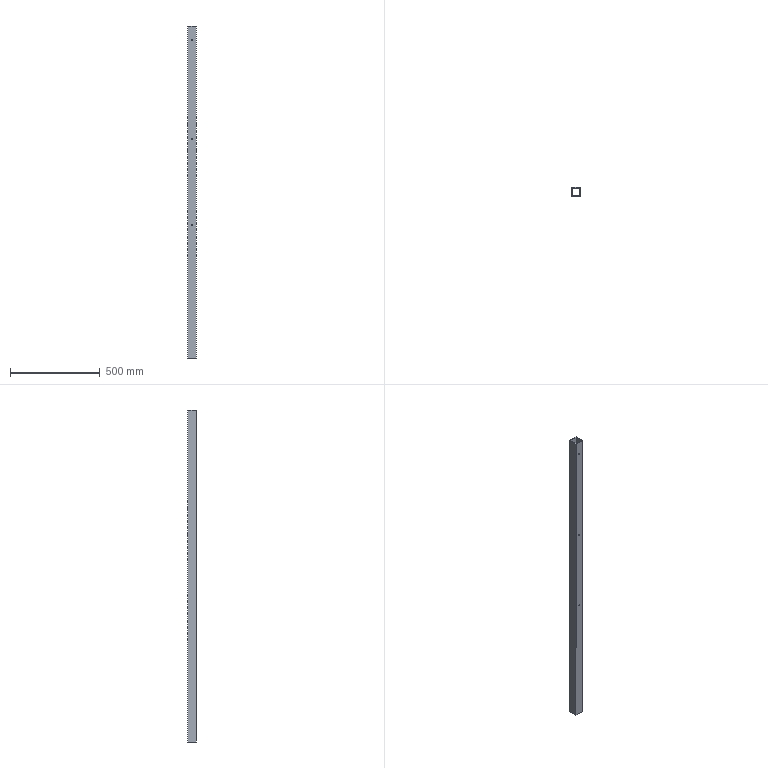Part | NX | features solid 2 | 1 solid | 16 faces | box 50 x 50 x 1848 mm | volume 1662776 mm3 | plane 10 | cylinder 6 | commonest cylinder face diameters 6 x6
STEP:
#1=CARTESIAN_POINT('',(-355.,5.,132.));
#2=VERTEX_POINT('',#1);
#3=CARTESIAN_POINT('',(-355.,0.,132.));
#4=VERTEX_POINT('',#3);
#5=CARTESIAN_POINT('',(-355.,1811.381,132.));
#6=DIRECTION('',(0.,-1.,0.));
#7=VECTOR('',#6,1000.);
#8=LINE('',#5,#7);
#9=EDGE_CURVE('',#2,#4,#8,.T.);
#10=ORIENTED_EDGE('',*,*,#9,.F.);
#11=CARTESIAN_POINT('',(-355.,5.,138.));
#12=VERTEX_POINT('',#11);
#13=CARTESIAN_POINT('',(-355.,5.,135.));
#14=DIRECTION('',(0.,1.,0.));
#15=DIRECTION('',(0.,0.,-1.));
#16=AXIS2_PLACEMENT_3D('',#13,#14,#15);
#17=CIRCLE('',#16,3.);
#18=EDGE_CURVE('',#2,#12,#17,.T.);
#19=ORIENTED_EDGE('',*,*,#18,.T.);
#20=CARTESIAN_POINT('',(-355.,0.,138.));
#21=VERTEX_POINT('',#20);
#22=CARTESIAN_POINT('',(-355.,1811.381,138.));
#23=DIRECTION('',(0.,-1.,0.));
#24=VECTOR('',#23,1000.);
#25=LINE('',#22,#24);
#26=EDGE_CURVE('',#21,#12,#25,.F.);
#27=ORIENTED_EDGE('',*,*,#26,.F.);
#28=CARTESIAN_POINT('',(-355.,0.,135.));
#29=DIRECTION('',(0.,-1.,0.));
#30=DIRECTION('',(0.,0.,1.));
#31=AXIS2_PLACEMENT_3D('',#28,#29,#30);
#32=CIRCLE('',#31,3.);
#33=EDGE_CURVE('',#21,#4,#32,.T.);
#34=ORIENTED_EDGE('',*,*,#33,.T.);
#35=EDGE_LOOP('',(#10,#19,#27,#34));
#36=FACE_BOUND('',#35,.T.);
#37=CARTESIAN_POINT('',(-355.,1811.381,135.));
#38=DIRECTION('',(0.,-1.,0.));
#39=DIRECTION('',(0.,0.,1.));
#40=AXIS2_PLACEMENT_3D('',#37,#38,#39);
#41=CYLINDRICAL_SURFACE('',#40,3.);
#42=ADVANCED_FACE('',(#36),#41,.F.);
#43=CARTESIAN_POINT('',(-355.,5.,612.));
#44=VERTEX_POINT('',#43);
#45=CARTESIAN_POINT('',(-355.,0.,612.));
#46=VERTEX_POINT('',#45);
#47=CARTESIAN_POINT('',(-355.,1811.381,612.));
#48=DIRECTION('',(0.,-1.,0.));
#49=VECTOR('',#48,1000.);
#50=LINE('',#47,#49);
#51=EDGE_CURVE('',#44,#46,#50,.T.);
#52=ORIENTED_EDGE('',*,*,#51,.F.);
#53=CARTESIAN_POINT('',(-355.,5.,618.));
#54=VERTEX_POINT('',#53);
#55=CARTESIAN_POINT('',(-355.,5.,615.));
#56=DIRECTION('',(0.,1.,0.));
#57=DIRECTION('',(0.,0.,-1.));
#58=AXIS2_PLACEMENT_3D('',#55,#56,#57);
#59=CIRCLE('',#58,3.);
#60=EDGE_CURVE('',#44,#54,#59,.T.);
#61=ORIENTED_EDGE('',*,*,#60,.T.);
#62=CARTESIAN_POINT('',(-355.,0.,618.));
#63=VERTEX_POINT('',#62);
#64=CARTESIAN_POINT('',(-355.,1811.381,618.));
#65=DIRECTION('',(0.,-1.,0.));
#66=VECTOR('',#65,1000.);
#67=LINE('',#64,#66);
#68=EDGE_CURVE('',#63,#54,#67,.F.);
#69=ORIENTED_EDGE('',*,*,#68,.F.);
#70=CARTESIAN_POINT('',(-355.,0.,615.));
#71=DIRECTION('',(0.,-1.,0.));
#72=DIRECTION('',(0.,0.,1.));
#73=AXIS2_PLACEMENT_3D('',#70,#71,#72);
#74=CIRCLE('',#73,3.);
#75=EDGE_CURVE('',#63,#46,#74,.T.);
#76=ORIENTED_EDGE('',*,*,#75,.T.);
#77=EDGE_LOOP('',(#52,#61,#69,#76));
#78=FACE_BOUND('',#77,.T.);
#79=CARTESIAN_POINT('',(-355.,1811.381,615.));
#80=DIRECTION('',(0.,-1.,0.));
#81=DIRECTION('',(0.,0.,1.));
#82=AXIS2_PLACEMENT_3D('',#79,#80,#81);
#83=CYLINDRICAL_SURFACE('',#82,3.);
#84=ADVANCED_FACE('',(#78),#83,.F.);
#85=CARTESIAN_POINT('',(-355.,0.,1162.));
#86=VERTEX_POINT('',#85);
#87=CARTESIAN_POINT('',(-355.,5.,1162.));
#88=VERTEX_POINT('',#87);
#89=CARTESIAN_POINT('',(-355.,1811.381,1162.));
#90=DIRECTION('',(0.,-1.,0.));
#91=VECTOR('',#90,1000.);
#92=LINE('',#89,#91);
#93=EDGE_CURVE('',#86,#88,#92,.F.);
#94=ORIENTED_EDGE('',*,*,#93,.T.);
#95=CARTESIAN_POINT('',(-355.,5.,1168.));
#96=VERTEX_POINT('',#95);
#97=CARTESIAN_POINT('',(-355.,5.,1165.));
#98=DIRECTION('',(0.,1.,0.));
#99=DIRECTION('',(0.,0.,-1.));
#100=AXIS2_PLACEMENT_3D('',#97,#98,#99);
#101=CIRCLE('',#100,3.);
#102=EDGE_CURVE('',#88,#96,#101,.T.);
#103=ORIENTED_EDGE('',*,*,#102,.T.);
#104=CARTESIAN_POINT('',(-355.,0.,1168.));
#105=VERTEX_POINT('',#104);
#106=CARTESIAN_POINT('',(-355.,1811.381,1168.));
#107=DIRECTION('',(0.,-1.,0.));
#108=VECTOR('',#107,1000.);
#109=LINE('',#106,#108);
#110=EDGE_CURVE('',#96,#105,#109,.T.);
#111=ORIENTED_EDGE('',*,*,#110,.T.);
#112=CARTESIAN_POINT('',(-355.,0.,1165.));
#113=DIRECTION('',(0.,-1.,0.));
#114=DIRECTION('',(0.,0.,1.));
#115=AXIS2_PLACEMENT_3D('',#112,#113,#114);
#116=CIRCLE('',#115,3.);
#117=EDGE_CURVE('',#105,#86,#116,.T.);
#118=ORIENTED_EDGE('',*,*,#117,.T.);
#119=EDGE_LOOP('',(#94,#103,#111,#118));
#120=FACE_BOUND('',#119,.T.);
#121=CARTESIAN_POINT('',(-355.,1811.381,1165.));
#122=DIRECTION('',(0.,-1.,0.));
#123=DIRECTION('',(0.,0.,1.));
#124=AXIS2_PLACEMENT_3D('',#121,#122,#123);
#125=CYLINDRICAL_SURFACE('',#124,3.);
#126=ADVANCED_FACE('',(#120),#125,.F.);
#127=CARTESIAN_POINT('',(-380.,50.,-603.));
#128=VERTEX_POINT('',#127);
#129=CARTESIAN_POINT('',(-380.,50.,1245.));
#130=VERTEX_POINT('',#129);
#131=CARTESIAN_POINT('',(-380.,50.,-495.));
#132=DIRECTION('',(0.,0.,1.));
#133=VECTOR('',#132,1000.);
#134=LINE('',#131,#133);
#135=EDGE_CURVE('',#128,#130,#134,.T.);
#136=ORIENTED_EDGE('',*,*,#135,.T.);
#137=CARTESIAN_POINT('',(-330.,50.,1245.));
#138=VERTEX_POINT('',#137);
#139=CARTESIAN_POINT('',(-380.,50.,1245.));
#140=DIRECTION('',(-1.,0.,0.));
#141=VECTOR('',#140,1000.);
#142=LINE('',#139,#141);
#143=EDGE_CURVE('',#138,#130,#142,.T.);
#144=ORIENTED_EDGE('',*,*,#143,.F.);
#145=CARTESIAN_POINT('',(-330.,50.,-603.));
#146=VERTEX_POINT('',#145);
#147=CARTESIAN_POINT('',(-330.,50.,-495.));
#148=DIRECTION('',(0.,0.,-1.));
#149=VECTOR('',#148,1000.);
#150=LINE('',#147,#149);
#151=EDGE_CURVE('',#138,#146,#150,.T.);
#152=ORIENTED_EDGE('',*,*,#151,.T.);
#153=CARTESIAN_POINT('',(-380.,50.,-603.));
#154=DIRECTION('',(-1.,0.,0.));
#155=VECTOR('',#154,1000.);
#156=LINE('',#153,#155);
#157=EDGE_CURVE('',#146,#128,#156,.T.);
#158=ORIENTED_EDGE('',*,*,#157,.T.);
#159=EDGE_LOOP('',(#136,#144,#152,#158));
#160=FACE_BOUND('',#159,.T.);
#161=CARTESIAN_POINT('',(-380.,50.,-495.));
#162=DIRECTION('',(0.,-1.,0.));
#163=DIRECTION('',(-1.,0.,0.));
#164=AXIS2_PLACEMENT_3D('',#161,#162,#163);
#165=PLANE('',#164);
#166=ADVANCED_FACE('',(#160),#165,.F.);
#167=CARTESIAN_POINT('',(-375.,45.,1245.));
#168=VERTEX_POINT('',#167);
#169=CARTESIAN_POINT('',(-335.,45.,1245.));
#170=VERTEX_POINT('',#169);
#171=CARTESIAN_POINT('',(-330.,45.,1245.));
#172=DIRECTION('',(1.,0.,0.));
#173=VECTOR('',#172,1000.);
#174=LINE('',#171,#173);
#175=EDGE_CURVE('',#168,#170,#174,.T.);
#176=ORIENTED_EDGE('',*,*,#175,.F.);
#177=CARTESIAN_POINT('',(-375.,45.,-603.));
#178=VERTEX_POINT('',#177);
#179=CARTESIAN_POINT('',(-375.,45.,-495.));
#180=DIRECTION('',(0.,0.,1.));
#181=VECTOR('',#180,1000.);
#182=LINE('',#179,#181);
#183=EDGE_CURVE('',#178,#168,#182,.T.);
#184=ORIENTED_EDGE('',*,*,#183,.F.);
#185=CARTESIAN_POINT('',(-335.,45.,-603.));
#186=VERTEX_POINT('',#185);
#187=CARTESIAN_POINT('',(-330.,45.,-603.));
#188=DIRECTION('',(1.,0.,0.));
#189=VECTOR('',#188,1000.);
#190=LINE('',#187,#189);
#191=EDGE_CURVE('',#178,#186,#190,.T.);
#192=ORIENTED_EDGE('',*,*,#191,.T.);
#193=CARTESIAN_POINT('',(-335.,45.,-495.));
#194=DIRECTION('',(0.,0.,-1.));
#195=VECTOR('',#194,1000.);
#196=LINE('',#193,#195);
#197=EDGE_CURVE('',#170,#186,#196,.T.);
#198=ORIENTED_EDGE('',*,*,#197,.F.);
#199=EDGE_LOOP('',(#176,#184,#192,#198));
#200=FACE_BOUND('',#199,.T.);
#201=CARTESIAN_POINT('',(-375.,45.,-495.));
#202=DIRECTION('',(0.,-1.,0.));
#203=DIRECTION('',(-1.,0.,0.));
#204=AXIS2_PLACEMENT_3D('',#201,#202,#203);
#205=PLANE('',#204);
#206=ADVANCED_FACE('',(#200),#205,.T.);
#207=CARTESIAN_POINT('',(-380.,0.,-603.));
#208=VERTEX_POINT('',#207);
#209=CARTESIAN_POINT('',(-380.,0.,1245.));
#210=VERTEX_POINT('',#209);
#211=CARTESIAN_POINT('',(-380.,0.,1245.));
#212=DIRECTION('',(0.,0.,1.));
#213=VECTOR('',#212,1000.);
#214=LINE('',#211,#213);
#215=EDGE_CURVE('',#208,#210,#214,.T.);
#216=ORIENTED_EDGE('',*,*,#215,.T.);
#217=CARTESIAN_POINT('',(-380.,0.,1245.));
#218=DIRECTION('',(0.,-1.,0.));
#219=VECTOR('',#218,1000.);
#220=LINE('',#217,#219);
#221=EDGE_CURVE('',#130,#210,#220,.T.);
#222=ORIENTED_EDGE('',*,*,#221,.F.);
#223=ORIENTED_EDGE('',*,*,#135,.F.);
#224=CARTESIAN_POINT('',(-380.,0.,-603.));
#225=DIRECTION('',(0.,-1.,0.));
#226=VECTOR('',#225,1000.);
#227=LINE('',#224,#226);
#228=EDGE_CURVE('',#128,#208,#227,.T.);
#229=ORIENTED_EDGE('',*,*,#228,.T.);
#230=EDGE_LOOP('',(#216,#222,#223,#229));
#231=FACE_BOUND('',#230,.T.);
#232=CARTESIAN_POINT('',(-380.,0.,1245.));
#233=DIRECTION('',(1.,0.,0.));
#234=DIRECTION('',(0.,-1.,0.));
#235=AXIS2_PLACEMENT_3D('',#232,#233,#234);
#236=PLANE('',#235);
#237=ADVANCED_FACE('',(#231),#236,.F.);
#238=ORIENTED_EDGE('',*,*,#151,.F.);
#239=CARTESIAN_POINT('',(-330.,0.,1245.));
#240=VERTEX_POINT('',#239);
#241=CARTESIAN_POINT('',(-330.,0.,1245.));
#242=DIRECTION('',(0.,1.,0.));
#243=VECTOR('',#242,1000.);
#244=LINE('',#241,#243);
#245=EDGE_CURVE('',#240,#138,#244,.T.);
#246=ORIENTED_EDGE('',*,*,#245,.F.);
#247=CARTESIAN_POINT('',(-330.,0.,-603.));
#248=VERTEX_POINT('',#247);
#249=CARTESIAN_POINT('',(-330.,0.,-495.));
#250=DIRECTION('',(0.,0.,-1.));
#251=VECTOR('',#250,1000.);
#252=LINE('',#249,#251);
#253=EDGE_CURVE('',#240,#248,#252,.T.);
#254=ORIENTED_EDGE('',*,*,#253,.T.);
#255=CARTESIAN_POINT('',(-330.,0.,-603.));
#256=DIRECTION('',(0.,1.,0.));
#257=VECTOR('',#256,1000.);
#258=LINE('',#255,#257);
#259=EDGE_CURVE('',#248,#146,#258,.T.);
#260=ORIENTED_EDGE('',*,*,#259,.T.);
#261=EDGE_LOOP('',(#238,#246,#254,#260));
#262=FACE_BOUND('',#261,.T.);
#263=CARTESIAN_POINT('',(-330.,0.,-495.));
#264=DIRECTION('',(-1.,0.,0.));
#265=DIRECTION('',(0.,0.,1.));
#266=AXIS2_PLACEMENT_3D('',#263,#264,#265);
#267=PLANE('',#266);
#268=ADVANCED_FACE('',(#262),#267,.F.);
#269=CARTESIAN_POINT('',(-335.,5.,-603.));
#270=VERTEX_POINT('',#269);
#271=CARTESIAN_POINT('',(-335.,0.,-603.));
#272=DIRECTION('',(0.,-1.,0.));
#273=VECTOR('',#272,1000.);
#274=LINE('',#271,#273);
#275=EDGE_CURVE('',#186,#270,#274,.T.);
#276=ORIENTED_EDGE('',*,*,#275,.F.);
#277=ORIENTED_EDGE('',*,*,#191,.F.);
#278=CARTESIAN_POINT('',(-375.,5.,-603.));
#279=VERTEX_POINT('',#278);
#280=CARTESIAN_POINT('',(-375.,0.,-603.));
#281=DIRECTION('',(0.,1.,0.));
#282=VECTOR('',#281,1000.);
#283=LINE('',#280,#282);
#284=EDGE_CURVE('',#279,#178,#283,.T.);
#285=ORIENTED_EDGE('',*,*,#284,.F.);
#286=CARTESIAN_POINT('',(-330.,5.,-603.));
#287=DIRECTION('',(-1.,0.,0.));
#288=VECTOR('',#287,1000.);
#289=LINE('',#286,#288);
#290=EDGE_CURVE('',#270,#279,#289,.T.);
#291=ORIENTED_EDGE('',*,*,#290,.F.);
#292=EDGE_LOOP('',(#276,#277,#285,#291));
#293=FACE_BOUND('',#292,.T.);
#294=ORIENTED_EDGE('',*,*,#228,.F.);
#295=ORIENTED_EDGE('',*,*,#157,.F.);
#296=ORIENTED_EDGE('',*,*,#259,.F.);
#297=CARTESIAN_POINT('',(-330.,0.,-603.));
#298=DIRECTION('',(-1.,0.,0.));
#299=VECTOR('',#298,1000.);
#300=LINE('',#297,#299);
#301=EDGE_CURVE('',#248,#208,#300,.T.);
#302=ORIENTED_EDGE('',*,*,#301,.T.);
#303=EDGE_LOOP('',(#294,#295,#296,#302));
#304=FACE_BOUND('',#303,.T.);
#305=CARTESIAN_POINT('',(-330.,0.,-603.));
#306=DIRECTION('',(0.,0.,1.));
#307=DIRECTION('',(0.,-1.,0.));
#308=AXIS2_PLACEMENT_3D('',#305,#306,#307);
#309=PLANE('',#308);
#310=ADVANCED_FACE('',(#293,#304),#309,.F.);
#311=CARTESIAN_POINT('',(-375.,5.,1245.));
#312=VERTEX_POINT('',#311);
#313=CARTESIAN_POINT('',(-375.,0.,1245.));
#314=DIRECTION('',(0.,1.,0.));
#315=VECTOR('',#314,1000.);
#316=LINE('',#313,#315);
#317=EDGE_CURVE('',#312,#168,#316,.T.);
#318=ORIENTED_EDGE('',*,*,#317,.F.);
#319=CARTESIAN_POINT('',(-375.,5.,1245.));
#320=DIRECTION('',(0.,0.,1.));
#321=VECTOR('',#320,1000.);
#322=LINE('',#319,#321);
#323=EDGE_CURVE('',#279,#312,#322,.T.);
#324=ORIENTED_EDGE('',*,*,#323,.F.);
#325=ORIENTED_EDGE('',*,*,#284,.T.);
#326=ORIENTED_EDGE('',*,*,#183,.T.);
#327=EDGE_LOOP('',(#318,#324,#325,#326));
#328=FACE_BOUND('',#327,.T.);
#329=CARTESIAN_POINT('',(-375.,5.,1245.));
#330=DIRECTION('',(1.,0.,0.));
#331=DIRECTION('',(0.,-1.,0.));
#332=AXIS2_PLACEMENT_3D('',#329,#330,#331);
#333=PLANE('',#332);
#334=ADVANCED_FACE('',(#328),#333,.T.);
#335=ORIENTED_EDGE('',*,*,#317,.T.);
#336=ORIENTED_EDGE('',*,*,#175,.T.);
#337=CARTESIAN_POINT('',(-335.,5.,1245.));
#338=VERTEX_POINT('',#337);
#339=CARTESIAN_POINT('',(-335.,45.,1245.));
#340=DIRECTION('',(0.,1.,0.));
#341=VECTOR('',#340,1000.);
#342=LINE('',#339,#341);
#343=EDGE_CURVE('',#338,#170,#342,.T.);
#344=ORIENTED_EDGE('',*,*,#343,.F.);
#345=CARTESIAN_POINT('',(-335.,5.,1245.));
#346=DIRECTION('',(1.,0.,0.));
#347=VECTOR('',#346,1000.);
#348=LINE('',#345,#347);
#349=EDGE_CURVE('',#312,#338,#348,.T.);
#350=ORIENTED_EDGE('',*,*,#349,.F.);
#351=EDGE_LOOP('',(#335,#336,#344,#350));
#352=FACE_BOUND('',#351,.T.);
#353=ORIENTED_EDGE('',*,*,#143,.T.);
#354=ORIENTED_EDGE('',*,*,#221,.T.);
#355=CARTESIAN_POINT('',(-330.,0.,1245.));
#356=DIRECTION('',(1.,0.,0.));
#357=VECTOR('',#356,1000.);
#358=LINE('',#355,#357);
#359=EDGE_CURVE('',#210,#240,#358,.T.);
#360=ORIENTED_EDGE('',*,*,#359,.T.);
#361=ORIENTED_EDGE('',*,*,#245,.T.);
#362=EDGE_LOOP('',(#353,#354,#360,#361));
#363=FACE_BOUND('',#362,.T.);
#364=CARTESIAN_POINT('',(-330.,0.,1245.));
#365=DIRECTION('',(0.,0.,1.));
#366=DIRECTION('',(0.,-1.,0.));
#367=AXIS2_PLACEMENT_3D('',#364,#365,#366);
#368=PLANE('',#367);
#369=ADVANCED_FACE('',(#352,#363),#368,.T.);
#370=ORIENTED_EDGE('',*,*,#343,.T.);
#371=ORIENTED_EDGE('',*,*,#197,.T.);
#372=ORIENTED_EDGE('',*,*,#275,.T.);
#373=CARTESIAN_POINT('',(-335.,5.,-495.));
#374=DIRECTION('',(0.,0.,-1.));
#375=VECTOR('',#374,1000.);
#376=LINE('',#373,#375);
#377=EDGE_CURVE('',#338,#270,#376,.T.);
#378=ORIENTED_EDGE('',*,*,#377,.F.);
#379=EDGE_LOOP('',(#370,#371,#372,#378));
#380=FACE_BOUND('',#379,.T.);
#381=CARTESIAN_POINT('',(-335.,45.,-495.));
#382=DIRECTION('',(-1.,0.,0.));
#383=DIRECTION('',(0.,0.,1.));
#384=AXIS2_PLACEMENT_3D('',#381,#382,#383);
#385=PLANE('',#384);
#386=ADVANCED_FACE('',(#380),#385,.T.);
#387=ORIENTED_EDGE('',*,*,#117,.F.);
#388=CARTESIAN_POINT('',(-355.,0.,1165.));
#389=DIRECTION('',(0.,-1.,0.));
#390=DIRECTION('',(0.,0.,1.));
#391=AXIS2_PLACEMENT_3D('',#388,#389,#390);
#392=CIRCLE('',#391,3.);
#393=EDGE_CURVE('',#86,#105,#392,.T.);
#394=ORIENTED_EDGE('',*,*,#393,.F.);
#395=EDGE_LOOP('',(#387,#394));
#396=FACE_BOUND('',#395,.T.);
#397=ORIENTED_EDGE('',*,*,#75,.F.);
#398=CARTESIAN_POINT('',(-355.,0.,615.));
#399=DIRECTION('',(0.,-1.,0.));
#400=DIRECTION('',(0.,0.,1.));
#401=AXIS2_PLACEMENT_3D('',#398,#399,#400);
#402=CIRCLE('',#401,3.);
#403=EDGE_CURVE('',#46,#63,#402,.T.);
#404=ORIENTED_EDGE('',*,*,#403,.F.);
#405=EDGE_LOOP('',(#397,#404));
#406=FACE_BOUND('',#405,.T.);
#407=ORIENTED_EDGE('',*,*,#33,.F.);
#408=CARTESIAN_POINT('',(-355.,0.,135.));
#409=DIRECTION('',(0.,-1.,0.));
#410=DIRECTION('',(0.,0.,1.));
#411=AXIS2_PLACEMENT_3D('',#408,#409,#410);
#412=CIRCLE('',#411,3.);
#413=EDGE_CURVE('',#4,#21,#412,.T.);
#414=ORIENTED_EDGE('',*,*,#413,.F.);
#415=EDGE_LOOP('',(#407,#414));
#416=FACE_BOUND('',#415,.T.);
#417=ORIENTED_EDGE('',*,*,#253,.F.);
#418=ORIENTED_EDGE('',*,*,#359,.F.);
#419=ORIENTED_EDGE('',*,*,#215,.F.);
#420=ORIENTED_EDGE('',*,*,#301,.F.);
#421=EDGE_LOOP('',(#417,#418,#419,#420));
#422=FACE_BOUND('',#421,.T.);
#423=CARTESIAN_POINT('',(-330.,0.,-495.));
#424=DIRECTION('',(0.,1.,0.));
#425=DIRECTION('',(1.,0.,0.));
#426=AXIS2_PLACEMENT_3D('',#423,#424,#425);
#427=PLANE('',#426);
#428=ADVANCED_FACE('',(#396,#406,#416,#422),#427,.F.);
#429=CARTESIAN_POINT('',(-355.,5.,1165.));
#430=DIRECTION('',(0.,1.,0.));
#431=DIRECTION('',(0.,0.,-1.));
#432=AXIS2_PLACEMENT_3D('',#429,#430,#431);
#433=CIRCLE('',#432,3.);
#434=EDGE_CURVE('',#96,#88,#433,.T.);
#435=ORIENTED_EDGE('',*,*,#434,.F.);
#436=ORIENTED_EDGE('',*,*,#102,.F.);
#437=EDGE_LOOP('',(#435,#436));
#438=FACE_BOUND('',#437,.T.);
#439=CARTESIAN_POINT('',(-355.,5.,615.));
#440=DIRECTION('',(0.,1.,0.));
#441=DIRECTION('',(0.,0.,-1.));
#442=AXIS2_PLACEMENT_3D('',#439,#440,#441);
#443=CIRCLE('',#442,3.);
#444=EDGE_CURVE('',#54,#44,#443,.T.);
#445=ORIENTED_EDGE('',*,*,#444,.F.);
#446=ORIENTED_EDGE('',*,*,#60,.F.);
#447=EDGE_LOOP('',(#445,#446));
#448=FACE_BOUND('',#447,.T.);
#449=CARTESIAN_POINT('',(-355.,5.,135.));
#450=DIRECTION('',(0.,1.,0.));
#451=DIRECTION('',(0.,0.,-1.));
#452=AXIS2_PLACEMENT_3D('',#449,#450,#451);
#453=CIRCLE('',#452,3.);
#454=EDGE_CURVE('',#12,#2,#453,.T.);
#455=ORIENTED_EDGE('',*,*,#454,.F.);
#456=ORIENTED_EDGE('',*,*,#18,.F.);
#457=EDGE_LOOP('',(#455,#456));
#458=FACE_BOUND('',#457,.T.);
#459=ORIENTED_EDGE('',*,*,#349,.T.);
#460=ORIENTED_EDGE('',*,*,#377,.T.);
#461=ORIENTED_EDGE('',*,*,#290,.T.);
#462=ORIENTED_EDGE('',*,*,#323,.T.);
#463=EDGE_LOOP('',(#459,#460,#461,#462));
#464=FACE_BOUND('',#463,.T.);
#465=CARTESIAN_POINT('',(-335.,5.,1245.));
#466=DIRECTION('',(0.,1.,0.));
#467=DIRECTION('',(1.,0.,0.));
#468=AXIS2_PLACEMENT_3D('',#465,#466,#467);
#469=PLANE('',#468);
#470=ADVANCED_FACE('',(#438,#448,#458,#464),#469,.T.);
#471=ORIENTED_EDGE('',*,*,#434,.T.);
#472=ORIENTED_EDGE('',*,*,#93,.F.);
#473=ORIENTED_EDGE('',*,*,#393,.T.);
#474=ORIENTED_EDGE('',*,*,#110,.F.);
#475=EDGE_LOOP('',(#471,#472,#473,#474));
#476=FACE_BOUND('',#475,.T.);
#477=CARTESIAN_POINT('',(-355.,1811.381,1165.));
#478=DIRECTION('',(0.,-1.,0.));
#479=DIRECTION('',(0.,0.,1.));
#480=AXIS2_PLACEMENT_3D('',#477,#478,#479);
#481=CYLINDRICAL_SURFACE('',#480,3.);
#482=ADVANCED_FACE('',(#476),#481,.F.);
#483=ORIENTED_EDGE('',*,*,#444,.T.);
#484=ORIENTED_EDGE('',*,*,#51,.T.);
#485=ORIENTED_EDGE('',*,*,#403,.T.);
#486=ORIENTED_EDGE('',*,*,#68,.T.);
#487=EDGE_LOOP('',(#483,#484,#485,#486));
#488=FACE_BOUND('',#487,.T.);
#489=CARTESIAN_POINT('',(-355.,1811.381,615.));
#490=DIRECTION('',(0.,-1.,0.));
#491=DIRECTION('',(0.,0.,1.));
#492=AXIS2_PLACEMENT_3D('',#489,#490,#491);
#493=CYLINDRICAL_SURFACE('',#492,3.);
#494=ADVANCED_FACE('',(#488),#493,.F.);
#495=ORIENTED_EDGE('',*,*,#454,.T.);
#496=ORIENTED_EDGE('',*,*,#9,.T.);
#497=ORIENTED_EDGE('',*,*,#413,.T.);
#498=ORIENTED_EDGE('',*,*,#26,.T.);
#499=EDGE_LOOP('',(#495,#496,#497,#498));
#500=FACE_BOUND('',#499,.T.);
#501=CARTESIAN_POINT('',(-355.,1811.381,135.));
#502=DIRECTION('',(0.,-1.,0.));
#503=DIRECTION('',(0.,0.,1.));
#504=AXIS2_PLACEMENT_3D('',#501,#502,#503);
#505=CYLINDRICAL_SURFACE('',#504,3.);
#506=ADVANCED_FACE('',(#500),#505,.F.);
#507=CLOSED_SHELL('',(#42,#84,#126,#166,#206,#237,#268,#310,#334,#369,#386,#428,#470,#482,#494,#506));
#508=MANIFOLD_SOLID_BREP('',#507);
#509=(LENGTH_UNIT()NAMED_UNIT(*)SI_UNIT(.MILLI.,.METRE.));
#510=UNCERTAINTY_MEASURE_WITH_UNIT(LENGTH_MEASURE(0.00001),#509,'','');
#511=(NAMED_UNIT(*)PLANE_ANGLE_UNIT()SI_UNIT($,.RADIAN.));
#512=(NAMED_UNIT(*)SI_UNIT($,.STERADIAN.)SOLID_ANGLE_UNIT());
#513=(GEOMETRIC_REPRESENTATION_CONTEXT(3)GLOBAL_UNCERTAINTY_ASSIGNED_CONTEXT((#510))GLOBAL_UNIT_ASSIGNED_CONTEXT((#509,#511,#512))REPRESENTATION_CONTEXT('',''));
#514=ADVANCED_BREP_SHAPE_REPRESENTATION('',(#508),#513);